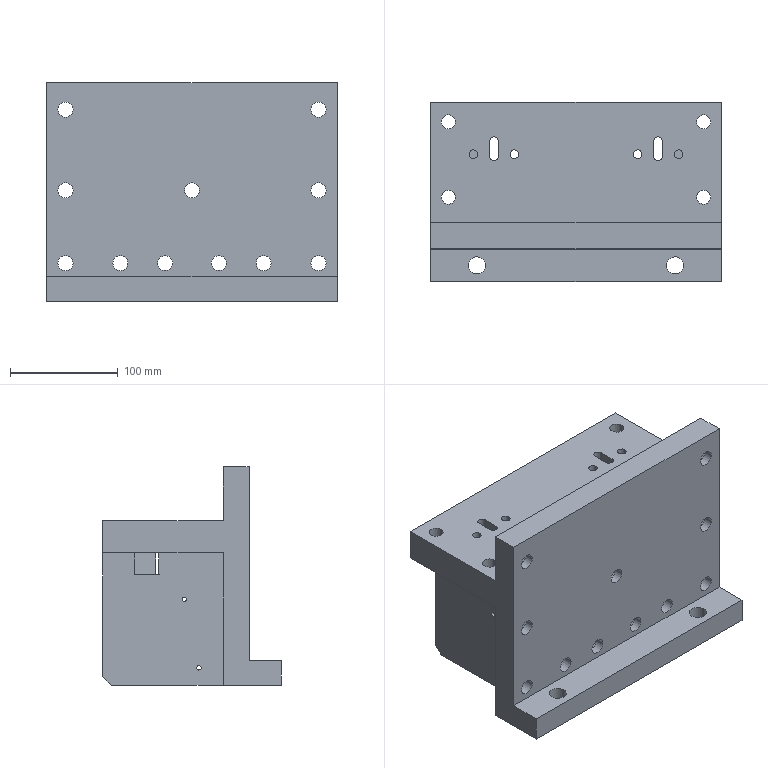Part | STEP file | GA KHUON COI GIUA.dwg | 1 solid | 105 faces | box 270 x 166 x 203 mm | volume 2828600 mm3 | cylinder 68 | plane 37 | commonest cylinder face diameters 14 x22 23 x14 8 x12 4.134 x8 13 x8 16 x4